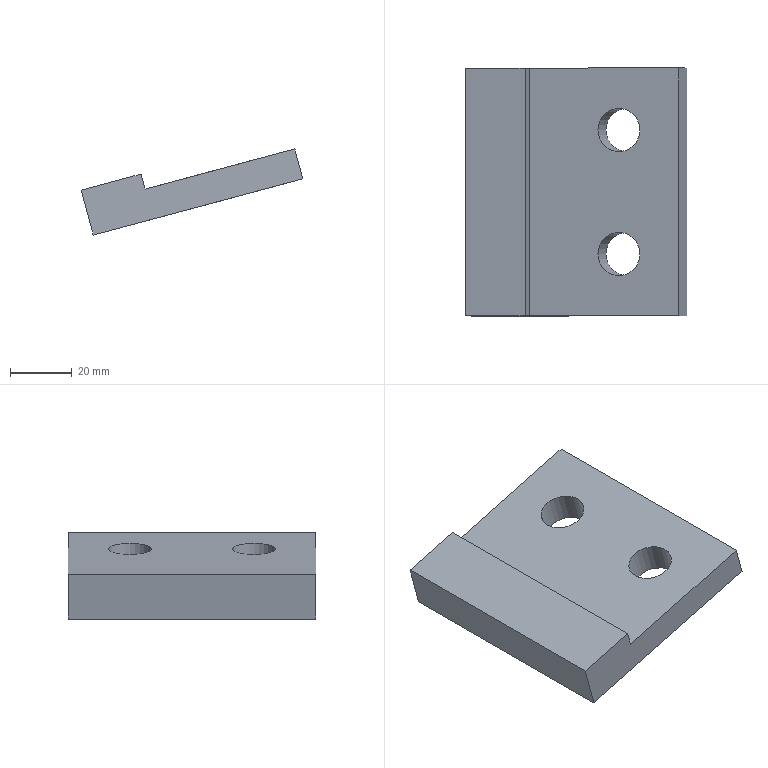Part | NX | features solid 2 | 1 solid | 10 faces | box 71.497 x 80 x 27.777 mm | volume 60921 mm3 | plane 8 | cylinder 2 | commonest cylinder face diameters 14 x2
STEP:
#1=CARTESIAN_POINT('',(713.947,-855.,-18.88));
#2=VERTEX_POINT('',#1);
#3=CARTESIAN_POINT('',(720.708,-855.,-17.069));
#4=DIRECTION('',(0.2588,0.,-0.9659));
#5=DIRECTION('',(-0.9659,0.,-0.2588));
#6=AXIS2_PLACEMENT_3D('',#3,#4,#5);
#7=CIRCLE('',#6,7.);
#8=EDGE_CURVE('',#2,#2,#7,.F.);
#9=ORIENTED_EDGE('',*,*,#8,.F.);
#10=EDGE_LOOP('',(#9));
#11=FACE_BOUND('',#10,.T.);
#12=CARTESIAN_POINT('',(691.73,-875.,-24.833));
#13=VERTEX_POINT('',#12);
#14=CARTESIAN_POINT('',(691.73,-795.,-24.833));
#15=VERTEX_POINT('',#14);
#16=CARTESIAN_POINT('',(691.73,-885.,-24.833));
#17=DIRECTION('',(0.,1.,0.));
#18=VECTOR('',#17,1000.);
#19=LINE('',#16,#18);
#20=EDGE_CURVE('',#13,#15,#19,.T.);
#21=ORIENTED_EDGE('',*,*,#20,.F.);
#22=CARTESIAN_POINT('',(740.027,-875.,-11.892));
#23=VERTEX_POINT('',#22);
#24=CARTESIAN_POINT('',(692.572,-875.,-24.608));
#25=DIRECTION('',(-0.9659,0.,-0.2588));
#26=VECTOR('',#25,1000.);
#27=LINE('',#24,#26);
#28=EDGE_CURVE('',#13,#23,#27,.F.);
#29=ORIENTED_EDGE('',*,*,#28,.T.);
#30=CARTESIAN_POINT('',(740.027,-795.,-11.892));
#31=VERTEX_POINT('',#30);
#32=CARTESIAN_POINT('',(740.027,-885.,-11.892));
#33=DIRECTION('',(0.,-1.,0.));
#34=VECTOR('',#33,1000.);
#35=LINE('',#32,#34);
#36=EDGE_CURVE('',#23,#31,#35,.F.);
#37=ORIENTED_EDGE('',*,*,#36,.T.);
#38=CARTESIAN_POINT('',(692.572,-795.,-24.608));
#39=DIRECTION('',(0.9659,0.,0.2588));
#40=VECTOR('',#39,1000.);
#41=LINE('',#38,#40);
#42=EDGE_CURVE('',#15,#31,#41,.T.);
#43=ORIENTED_EDGE('',*,*,#42,.F.);
#44=EDGE_LOOP('',(#21,#29,#37,#43));
#45=FACE_BOUND('',#44,.T.);
#46=CARTESIAN_POINT('',(713.947,-815.,-18.88));
#47=VERTEX_POINT('',#46);
#48=CARTESIAN_POINT('',(720.708,-815.,-17.069));
#49=DIRECTION('',(0.2588,0.,-0.9659));
#50=DIRECTION('',(-0.9659,0.,-0.2588));
#51=AXIS2_PLACEMENT_3D('',#48,#49,#50);
#52=CIRCLE('',#51,7.);
#53=EDGE_CURVE('',#47,#47,#52,.F.);
#54=ORIENTED_EDGE('',*,*,#53,.F.);
#55=EDGE_LOOP('',(#54));
#56=FACE_BOUND('',#55,.T.);
#57=CARTESIAN_POINT('',(692.572,-885.,-24.608));
#58=DIRECTION('',(0.2588,0.,-0.9659));
#59=DIRECTION('',(0.9659,0.,0.2588));
#60=AXIS2_PLACEMENT_3D('',#57,#58,#59);
#61=PLANE('',#60);
#62=ADVANCED_FACE('',(#11,#45,#56),#61,.F.);
#63=CARTESIAN_POINT('',(716.535,-855.,-28.54));
#64=VERTEX_POINT('',#63);
#65=CARTESIAN_POINT('',(723.296,-855.,-26.728));
#66=DIRECTION('',(0.2588,0.,-0.9659));
#67=DIRECTION('',(-0.9659,0.,-0.2588));
#68=AXIS2_PLACEMENT_3D('',#65,#66,#67);
#69=CIRCLE('',#68,7.);
#70=EDGE_CURVE('',#64,#64,#69,.F.);
#71=ORIENTED_EDGE('',*,*,#70,.T.);
#72=EDGE_LOOP('',(#71));
#73=FACE_BOUND('',#72,.T.);
#74=CARTESIAN_POINT('',(675.,-795.,-39.669));
#75=VERTEX_POINT('',#74);
#76=CARTESIAN_POINT('',(742.615,-795.,-21.552));
#77=VERTEX_POINT('',#76);
#78=CARTESIAN_POINT('',(695.16,-795.,-34.267));
#79=DIRECTION('',(0.9659,0.,0.2588));
#80=VECTOR('',#79,1000.);
#81=LINE('',#78,#80);
#82=EDGE_CURVE('',#75,#77,#81,.T.);
#83=ORIENTED_EDGE('',*,*,#82,.T.);
#84=CARTESIAN_POINT('',(742.615,-875.,-21.552));
#85=VERTEX_POINT('',#84);
#86=CARTESIAN_POINT('',(742.615,-885.,-21.552));
#87=DIRECTION('',(0.,-1.,0.));
#88=VECTOR('',#87,1000.);
#89=LINE('',#86,#88);
#90=EDGE_CURVE('',#85,#77,#89,.F.);
#91=ORIENTED_EDGE('',*,*,#90,.F.);
#92=CARTESIAN_POINT('',(675.,-875.,-39.669));
#93=VERTEX_POINT('',#92);
#94=CARTESIAN_POINT('',(695.16,-875.,-34.267));
#95=DIRECTION('',(-0.9659,0.,-0.2588));
#96=VECTOR('',#95,1000.);
#97=LINE('',#94,#96);
#98=EDGE_CURVE('',#93,#85,#97,.F.);
#99=ORIENTED_EDGE('',*,*,#98,.F.);
#100=CARTESIAN_POINT('',(675.,-885.,-39.669));
#101=DIRECTION('',(0.,1.,0.));
#102=VECTOR('',#101,1000.);
#103=LINE('',#100,#102);
#104=EDGE_CURVE('',#93,#75,#103,.T.);
#105=ORIENTED_EDGE('',*,*,#104,.T.);
#106=EDGE_LOOP('',(#83,#91,#99,#105));
#107=FACE_BOUND('',#106,.T.);
#108=CARTESIAN_POINT('',(716.535,-815.,-28.54));
#109=VERTEX_POINT('',#108);
#110=CARTESIAN_POINT('',(723.296,-815.,-26.728));
#111=DIRECTION('',(0.2588,0.,-0.9659));
#112=DIRECTION('',(-0.9659,0.,-0.2588));
#113=AXIS2_PLACEMENT_3D('',#110,#111,#112);
#114=CIRCLE('',#113,7.);
#115=EDGE_CURVE('',#109,#109,#114,.F.);
#116=ORIENTED_EDGE('',*,*,#115,.T.);
#117=EDGE_LOOP('',(#116));
#118=FACE_BOUND('',#117,.T.);
#119=CARTESIAN_POINT('',(695.16,-885.,-34.267));
#120=DIRECTION('',(0.2588,0.,-0.9659));
#121=DIRECTION('',(0.9659,0.,0.2588));
#122=AXIS2_PLACEMENT_3D('',#119,#120,#121);
#123=PLANE('',#122);
#124=ADVANCED_FACE('',(#73,#107,#118),#123,.T.);
#125=CARTESIAN_POINT('',(671.118,-795.,-25.18));
#126=VERTEX_POINT('',#125);
#127=CARTESIAN_POINT('',(690.436,-795.,-20.004));
#128=VERTEX_POINT('',#127);
#129=CARTESIAN_POINT('',(691.278,-795.,-19.778));
#130=DIRECTION('',(0.9659,0.,0.2588));
#131=VECTOR('',#130,1000.);
#132=LINE('',#129,#131);
#133=EDGE_CURVE('',#126,#128,#132,.T.);
#134=ORIENTED_EDGE('',*,*,#133,.F.);
#135=CARTESIAN_POINT('',(671.118,-875.,-25.18));
#136=VERTEX_POINT('',#135);
#137=CARTESIAN_POINT('',(671.118,-885.,-25.18));
#138=DIRECTION('',(0.,1.,0.));
#139=VECTOR('',#138,1000.);
#140=LINE('',#137,#139);
#141=EDGE_CURVE('',#136,#126,#140,.T.);
#142=ORIENTED_EDGE('',*,*,#141,.F.);
#143=CARTESIAN_POINT('',(690.436,-875.,-20.004));
#144=VERTEX_POINT('',#143);
#145=CARTESIAN_POINT('',(671.96,-875.,-24.954));
#146=DIRECTION('',(-0.9659,0.,-0.2588));
#147=VECTOR('',#146,1000.);
#148=LINE('',#145,#147);
#149=EDGE_CURVE('',#136,#144,#148,.F.);
#150=ORIENTED_EDGE('',*,*,#149,.T.);
#151=CARTESIAN_POINT('',(690.436,-885.,-20.004));
#152=DIRECTION('',(0.,1.,0.));
#153=VECTOR('',#152,1000.);
#154=LINE('',#151,#153);
#155=EDGE_CURVE('',#144,#128,#154,.T.);
#156=ORIENTED_EDGE('',*,*,#155,.T.);
#157=EDGE_LOOP('',(#134,#142,#150,#156));
#158=FACE_BOUND('',#157,.T.);
#159=CARTESIAN_POINT('',(671.96,-885.,-24.954));
#160=DIRECTION('',(0.2588,0.,-0.9659));
#161=DIRECTION('',(0.,1.,0.));
#162=AXIS2_PLACEMENT_3D('',#159,#160,#161);
#163=PLANE('',#162);
#164=ADVANCED_FACE('',(#158),#163,.F.);
#165=ORIENTED_EDGE('',*,*,#155,.F.);
#166=CARTESIAN_POINT('',(691.73,-875.,-24.833));
#167=DIRECTION('',(0.2588,0.,-0.9659));
#168=VECTOR('',#167,1000.);
#169=LINE('',#166,#168);
#170=EDGE_CURVE('',#13,#144,#169,.F.);
#171=ORIENTED_EDGE('',*,*,#170,.F.);
#172=ORIENTED_EDGE('',*,*,#20,.T.);
#173=CARTESIAN_POINT('',(691.73,-795.,-24.833));
#174=DIRECTION('',(-0.2588,0.,0.9659));
#175=VECTOR('',#174,1000.);
#176=LINE('',#173,#175);
#177=EDGE_CURVE('',#15,#128,#176,.T.);
#178=ORIENTED_EDGE('',*,*,#177,.T.);
#179=EDGE_LOOP('',(#165,#171,#172,#178));
#180=FACE_BOUND('',#179,.T.);
#181=CARTESIAN_POINT('',(691.73,-885.,-24.833));
#182=DIRECTION('',(-0.9659,0.,-0.2588));
#183=DIRECTION('',(0.2588,0.,-0.9659));
#184=AXIS2_PLACEMENT_3D('',#181,#182,#183);
#185=PLANE('',#184);
#186=ADVANCED_FACE('',(#180),#185,.F.);
#187=CARTESIAN_POINT('',(740.027,-875.,-11.892));
#188=DIRECTION('',(-0.2588,0.,0.9659));
#189=VECTOR('',#188,1000.);
#190=LINE('',#187,#189);
#191=EDGE_CURVE('',#85,#23,#190,.T.);
#192=ORIENTED_EDGE('',*,*,#191,.F.);
#193=ORIENTED_EDGE('',*,*,#90,.T.);
#194=CARTESIAN_POINT('',(730.978,-795.,21.878));
#195=DIRECTION('',(0.2588,0.,-0.9659));
#196=VECTOR('',#195,1000.);
#197=LINE('',#194,#196);
#198=EDGE_CURVE('',#77,#31,#197,.F.);
#199=ORIENTED_EDGE('',*,*,#198,.T.);
#200=ORIENTED_EDGE('',*,*,#36,.F.);
#201=EDGE_LOOP('',(#192,#193,#199,#200));
#202=FACE_BOUND('',#201,.T.);
#203=CARTESIAN_POINT('',(730.978,-889.636,21.878));
#204=DIRECTION('',(0.9659,0.,0.2588));
#205=DIRECTION('',(0.2588,0.,-0.9659));
#206=AXIS2_PLACEMENT_3D('',#203,#204,#205);
#207=PLANE('',#206);
#208=ADVANCED_FACE('',(#202),#207,.T.);
#209=CARTESIAN_POINT('',(672.412,-875.,-30.01));
#210=DIRECTION('',(0.2588,0.,-0.9659));
#211=VECTOR('',#210,1000.);
#212=LINE('',#209,#211);
#213=EDGE_CURVE('',#93,#136,#212,.F.);
#214=ORIENTED_EDGE('',*,*,#213,.F.);
#215=ORIENTED_EDGE('',*,*,#98,.T.);
#216=ORIENTED_EDGE('',*,*,#191,.T.);
#217=ORIENTED_EDGE('',*,*,#28,.F.);
#218=ORIENTED_EDGE('',*,*,#170,.T.);
#219=ORIENTED_EDGE('',*,*,#149,.F.);
#220=EDGE_LOOP('',(#214,#215,#216,#217,#218,#219));
#221=FACE_BOUND('',#220,.T.);
#222=CARTESIAN_POINT('',(692.572,-875.,-24.608));
#223=DIRECTION('',(0.,-1.,0.));
#224=DIRECTION('',(0.9659,0.,0.2588));
#225=AXIS2_PLACEMENT_3D('',#222,#223,#224);
#226=PLANE('',#225);
#227=ADVANCED_FACE('',(#221),#226,.T.);
#228=ORIENTED_EDGE('',*,*,#104,.F.);
#229=ORIENTED_EDGE('',*,*,#213,.T.);
#230=ORIENTED_EDGE('',*,*,#141,.T.);
#231=CARTESIAN_POINT('',(672.412,-795.,-30.01));
#232=DIRECTION('',(-0.2588,0.,0.9659));
#233=VECTOR('',#232,1000.);
#234=LINE('',#231,#233);
#235=EDGE_CURVE('',#75,#126,#234,.T.);
#236=ORIENTED_EDGE('',*,*,#235,.F.);
#237=EDGE_LOOP('',(#228,#229,#230,#236));
#238=FACE_BOUND('',#237,.T.);
#239=CARTESIAN_POINT('',(672.412,-885.,-30.01));
#240=DIRECTION('',(0.9659,0.,0.2588));
#241=DIRECTION('',(0.,1.,0.));
#242=AXIS2_PLACEMENT_3D('',#239,#240,#241);
#243=PLANE('',#242);
#244=ADVANCED_FACE('',(#238),#243,.F.);
#245=ORIENTED_EDGE('',*,*,#198,.F.);
#246=ORIENTED_EDGE('',*,*,#82,.F.);
#247=ORIENTED_EDGE('',*,*,#235,.T.);
#248=ORIENTED_EDGE('',*,*,#133,.T.);
#249=ORIENTED_EDGE('',*,*,#177,.F.);
#250=ORIENTED_EDGE('',*,*,#42,.T.);
#251=EDGE_LOOP('',(#245,#246,#247,#248,#249,#250));
#252=FACE_BOUND('',#251,.T.);
#253=CARTESIAN_POINT('',(692.572,-795.,-24.608));
#254=DIRECTION('',(0.,-1.,0.));
#255=DIRECTION('',(0.9659,0.,0.2588));
#256=AXIS2_PLACEMENT_3D('',#253,#254,#255);
#257=PLANE('',#256);
#258=ADVANCED_FACE('',(#252),#257,.F.);
#259=ORIENTED_EDGE('',*,*,#70,.F.);
#260=EDGE_LOOP('',(#259));
#261=FACE_BOUND('',#260,.T.);
#262=ORIENTED_EDGE('',*,*,#8,.T.);
#263=EDGE_LOOP('',(#262));
#264=FACE_BOUND('',#263,.T.);
#265=CARTESIAN_POINT('',(732.314,-855.,-60.381));
#266=DIRECTION('',(-0.2588,0.,0.9659));
#267=DIRECTION('',(-0.9659,0.,-0.2588));
#268=AXIS2_PLACEMENT_3D('',#265,#266,#267);
#269=CYLINDRICAL_SURFACE('',#268,7.);
#270=ADVANCED_FACE('',(#261,#264),#269,.F.);
#271=ORIENTED_EDGE('',*,*,#115,.F.);
#272=EDGE_LOOP('',(#271));
#273=FACE_BOUND('',#272,.T.);
#274=ORIENTED_EDGE('',*,*,#53,.T.);
#275=EDGE_LOOP('',(#274));
#276=FACE_BOUND('',#275,.T.);
#277=CARTESIAN_POINT('',(732.314,-815.,-60.381));
#278=DIRECTION('',(-0.2588,0.,0.9659));
#279=DIRECTION('',(-0.9659,0.,-0.2588));
#280=AXIS2_PLACEMENT_3D('',#277,#278,#279);
#281=CYLINDRICAL_SURFACE('',#280,7.);
#282=ADVANCED_FACE('',(#273,#276),#281,.F.);
#283=CLOSED_SHELL('',(#62,#124,#164,#186,#208,#227,#244,#258,#270,#282));
#284=MANIFOLD_SOLID_BREP('',#283);
#285=(LENGTH_UNIT()NAMED_UNIT(*)SI_UNIT(.MILLI.,.METRE.));
#286=UNCERTAINTY_MEASURE_WITH_UNIT(LENGTH_MEASURE(0.00001),#285,'','');
#287=(NAMED_UNIT(*)PLANE_ANGLE_UNIT()SI_UNIT($,.RADIAN.));
#288=(NAMED_UNIT(*)SI_UNIT($,.STERADIAN.)SOLID_ANGLE_UNIT());
#289=(GEOMETRIC_REPRESENTATION_CONTEXT(3)GLOBAL_UNCERTAINTY_ASSIGNED_CONTEXT((#286))GLOBAL_UNIT_ASSIGNED_CONTEXT((#285,#287,#288))REPRESENTATION_CONTEXT('',''));
#290=ADVANCED_BREP_SHAPE_REPRESENTATION('',(#284),#289);